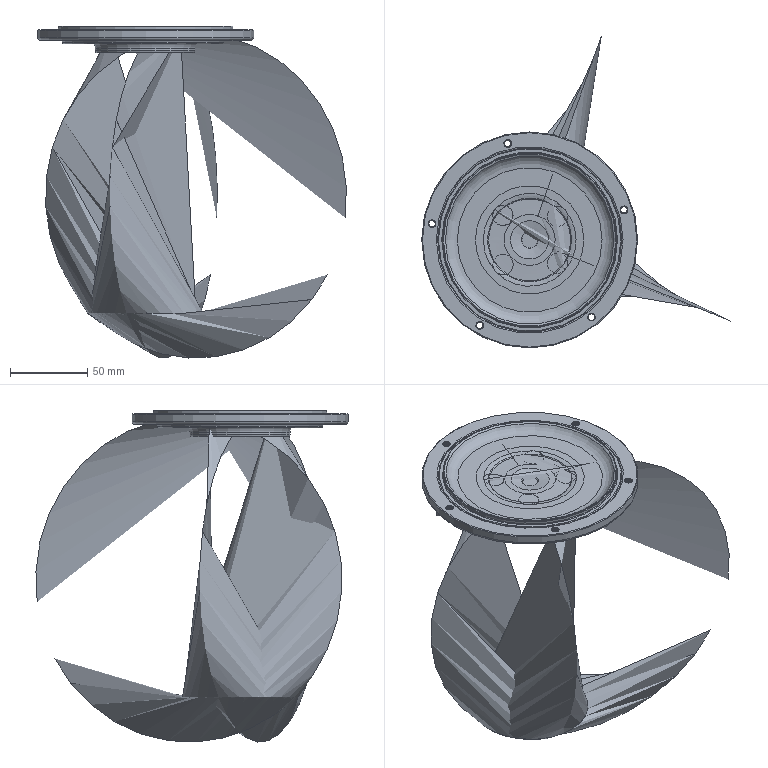NC program | NX | posted with a generic post
Lines 1954 to 2005 of 2005:
(PLANAR_MILL_COPY , TOOL : D6A45)
N3882 T07 M6
N3884 G54
N3886 G17 G0 G90 X15.399 Y-18.317 S9500 M3
N3888 G43 Z30. H7
N3890 Z-3.7
N3892 G94 G1 Z-5.2 F1500.
N3894 X15.01 Y-19.126
N3896 G3 X15.876 Y-19.626 R1.
N3898 X18.176 Y-17.326 R2.3
N3900 X15.876 Y-19.626 R-2.3
N3902 X16.742 Y-19.126 R1.
N3904 G1 X16.353 Y-18.317
N3906 Z-3.7
N3908 G0 Z30.
N3910 X-16.414 Y-18.262
N3912 Z-3.7
N3914 G1 Z-5.2
N3916 X-16.803 Y-19.07
N3918 G3 X-15.937 Y-19.57 R1.
N3920 X-13.637 Y-17.27 R2.3
N3922 X-15.937 Y-19.57 R-2.3
N3924 X-15.071 Y-19.07 R1.
N3926 G1 X-15.46 Y-18.262
N3928 Z-3.7
N3930 G0 Z30.
N3932 X-15.582 Y17.011
N3934 Z-3.7
N3936 G1 Z-5.2
N3938 X-15.972 Y16.202
N3940 G3 X-15.106 Y15.702 R1.
N3942 X-12.806 Y18.002 R2.3
N3944 X-15.106 Y15.702 R-2.3
N3946 X-14.239 Y16.202 R1.
N3948 G1 X-14.629 Y17.011
N3950 Z-3.7
N3952 G0 Z30.
N3954 X14.691 Y16.958
N3956 Z-3.7
N3958 G1 Z-5.2
N3960 X14.302 Y16.149
N3962 G3 X15.168 Y15.649 R1.
N3964 X17.468 Y17.949 R2.3
N3966 X15.168 Y15.649 R-2.3
N3968 X16.034 Y16.149 R1.
N3970 G1 X15.645 Y16.958
N3972 Z-3.7
N3974 G0 Z30.
N3976 M5
N3978 M2